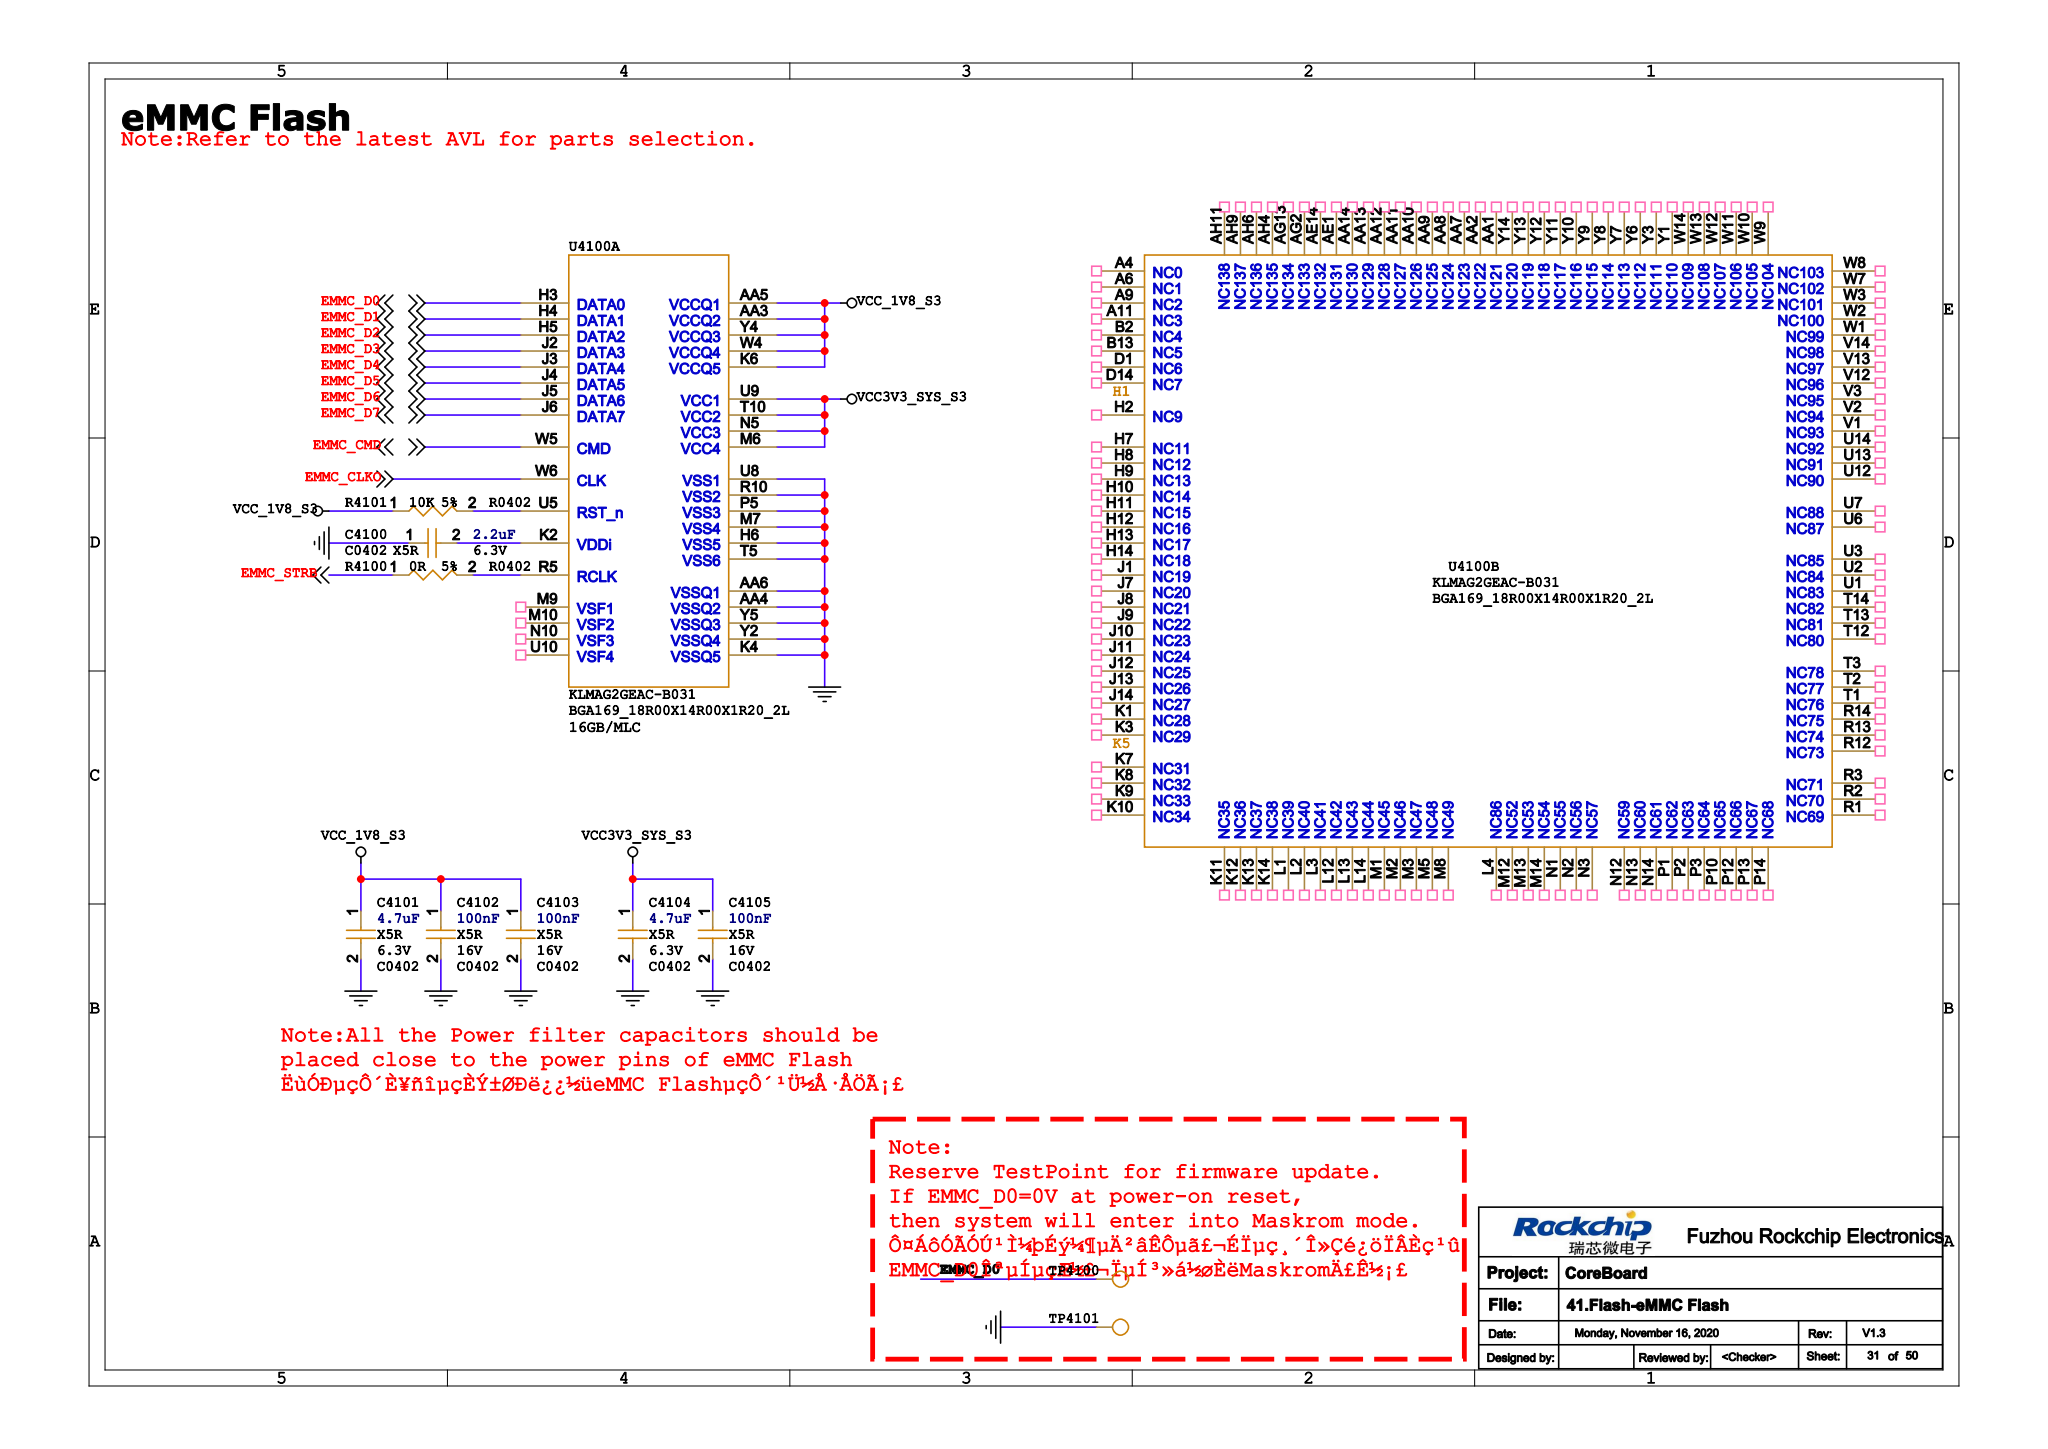Circuit board | Cadence Allegro | 749 parts | 717 nets | one sheet of the schematic
Parts on this sheet (reference | value | footprint):
C4100 | 2.2uF | C0402
C4101 | 4.7uF | C0402
C4102 | 100nF | C0402
C4103 | 100nF | C0402
C4104 | 4.7uF | C0402
C4105 | 100nF | C0402
TP4100 | TP_0.7 | TP_0R70
TP4101 | TP_0.7 | TP_0R70
U4100 | KLMAG2GEAC-B031 | BGA169_18R00X14R00X1R20_2L
Nets of these parts (net: part-pin ...):
GND: C4100-1 C4101-2 C4102-2 C4103-2 C4104-2 C4105-2 TP4101-1 U4100-AA4 U4100-AA6 U4100-H6 U4100-K4 U4100-M7 U4100-P5 U4100-R10 U4100-T5 U4100-U8 U4100-Y2 U4100-Y5
VCC3V3_SYS_S3: C4104-1 C4105-1 U4100-M6 U4100-N5 U4100-T10 U4100-U9
N74763326: C4100-2 U4100-K2
VCC_1V8_S3: C4101-1 C4102-1 C4103-1 U4100-AA3 U4100-AA5 U4100-K6 U4100-W4 U4100-Y4
EMMC_CMD: U4100-W5
EMMC_D0: TP4100-1 U4100-H3
EMMC_D1: U4100-H4
EMMC_D2: U4100-H5
EMMC_D3: U4100-J2
EMMC_D4: U4100-J3
EMMC_D5: U4100-J4
EMMC_D6: U4100-J5
EMMC_D7: U4100-J6
EMMC_CLKO: U4100-W6